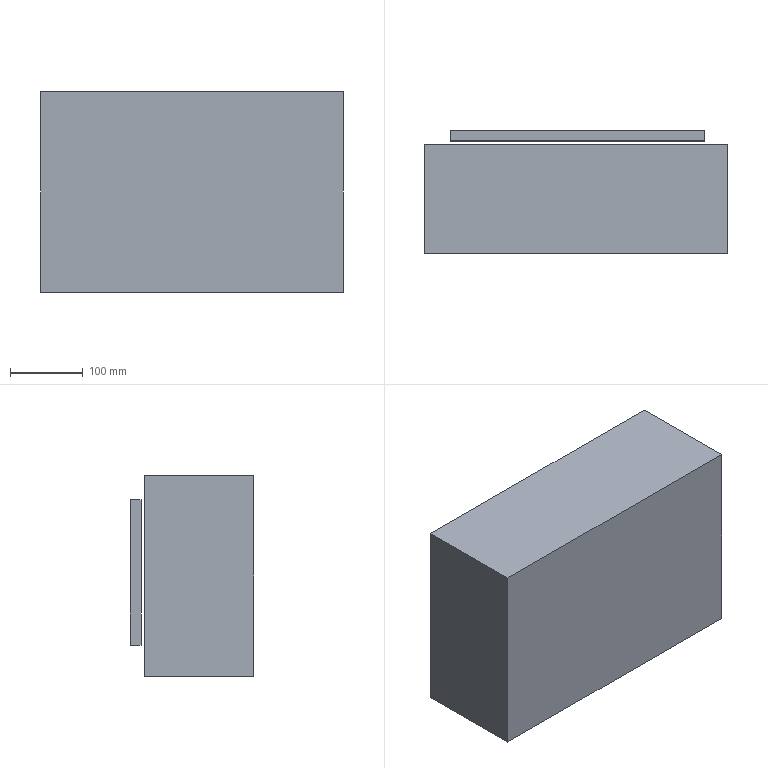Part | STEP file | Plate | 2 solids | 17 faces | box 416 x 170 x 276 mm | volume 18168400 mm3 | plane 17
STEP:
#1=CARTESIAN_POINT('',(0.,0.,0.));
#2=DIRECTION('',(0.,0.,1.));
#3=DIRECTION('',(1.,0.,0.));
#4=AXIS2_PLACEMENT_3D('',#1,#2,#3);
#5=CARTESIAN_POINT('',(238.509,-108.087,0.));
#6=VERTEX_POINT('',#5);
#7=CARTESIAN_POINT('',(238.509,41.913,0.));
#8=VERTEX_POINT('',#7);
#9=CARTESIAN_POINT('',(238.509,-108.087,0.));
#10=DIRECTION('',(0.,1.,0.));
#11=VECTOR('',#10,1.);
#12=LINE('',#9,#11);
#13=CARTESIAN_POINT('',(238.509,-108.087,-276.));
#14=DIRECTION('',(1.,0.,0.));
#15=DIRECTION('',(0.,0.,-1.));
#16=AXIS2_PLACEMENT_3D('',#13,#14,#15);
#17=PLANE('',#16);
#18=CARTESIAN_POINT('',(-276.,0.));
#19=DIRECTION('',(0.,1.));
#20=VECTOR('',#19,1.);
#21=LINE('',#18,#20);
#22=(GEOMETRIC_REPRESENTATION_CONTEXT(2)PARAMETRIC_REPRESENTATION_CONTEXT()REPRESENTATION_CONTEXT('',''));
#23=DEFINITIONAL_REPRESENTATION('',(#21),#22);
#24=PCURVE('',#17,#23);
#25=CARTESIAN_POINT('',(0.,0.,0.));
#26=DIRECTION('',(0.,0.,-1.));
#27=DIRECTION('',(-1.,0.,0.));
#28=AXIS2_PLACEMENT_3D('',#25,#26,#27);
#29=PLANE('',#28);
#30=CARTESIAN_POINT('',(-238.509,-108.087));
#31=DIRECTION('',(0.,1.));
#32=VECTOR('',#31,1.);
#33=LINE('',#30,#32);
#34=(GEOMETRIC_REPRESENTATION_CONTEXT(2)PARAMETRIC_REPRESENTATION_CONTEXT()REPRESENTATION_CONTEXT('',''));
#35=DEFINITIONAL_REPRESENTATION('',(#33),#34);
#36=PCURVE('',#29,#35);
#37=SURFACE_CURVE('',#12,(#24,#36),.PCURVE_S1.);
#38=EDGE_CURVE('',#6,#8,#37,.T.);
#39=ORIENTED_EDGE('',*,*,#38,.F.);
#40=CARTESIAN_POINT('',(238.509,-108.087,-276.));
#41=VERTEX_POINT('',#40);
#42=CARTESIAN_POINT('',(238.509,-108.087,-276.));
#43=DIRECTION('',(0.,0.,1.));
#44=VECTOR('',#43,1.);
#45=LINE('',#42,#44);
#46=CARTESIAN_POINT('',(0.,0.));
#47=DIRECTION('',(-1.,0.));
#48=VECTOR('',#47,1.);
#49=LINE('',#46,#48);
#50=(GEOMETRIC_REPRESENTATION_CONTEXT(2)PARAMETRIC_REPRESENTATION_CONTEXT()REPRESENTATION_CONTEXT('',''));
#51=DEFINITIONAL_REPRESENTATION('',(#49),#50);
#52=PCURVE('',#17,#51);
#53=CARTESIAN_POINT('',(-177.491,-108.087,-276.));
#54=DIRECTION('',(0.,-1.,0.));
#55=DIRECTION('',(0.,0.,-1.));
#56=AXIS2_PLACEMENT_3D('',#53,#54,#55);
#57=PLANE('',#56);
#58=CARTESIAN_POINT('',(0.,416.));
#59=DIRECTION('',(-1.,0.));
#60=VECTOR('',#59,1.);
#61=LINE('',#58,#60);
#62=(GEOMETRIC_REPRESENTATION_CONTEXT(2)PARAMETRIC_REPRESENTATION_CONTEXT()REPRESENTATION_CONTEXT('',''));
#63=DEFINITIONAL_REPRESENTATION('',(#61),#62);
#64=PCURVE('',#57,#63);
#65=SURFACE_CURVE('',#45,(#52,#64),.PCURVE_S1.);
#66=EDGE_CURVE('',#41,#6,#65,.T.);
#67=ORIENTED_EDGE('',*,*,#66,.F.);
#68=CARTESIAN_POINT('',(238.509,41.913,-276.));
#69=VERTEX_POINT('',#68);
#70=CARTESIAN_POINT('',(238.509,-108.087,-276.));
#71=DIRECTION('',(0.,1.,0.));
#72=VECTOR('',#71,1.);
#73=LINE('',#70,#72);
#74=CARTESIAN_POINT('',(0.,0.));
#75=DIRECTION('',(0.,1.));
#76=VECTOR('',#75,1.);
#77=LINE('',#74,#76);
#78=(GEOMETRIC_REPRESENTATION_CONTEXT(2)PARAMETRIC_REPRESENTATION_CONTEXT()REPRESENTATION_CONTEXT('',''));
#79=DEFINITIONAL_REPRESENTATION('',(#77),#78);
#80=PCURVE('',#17,#79);
#81=CARTESIAN_POINT('',(0.,0.,-276.));
#82=DIRECTION('',(0.,0.,-1.));
#83=DIRECTION('',(-1.,0.,0.));
#84=AXIS2_PLACEMENT_3D('',#81,#82,#83);
#85=PLANE('',#84);
#86=CARTESIAN_POINT('',(-238.509,-108.087));
#87=DIRECTION('',(0.,1.));
#88=VECTOR('',#87,1.);
#89=LINE('',#86,#88);
#90=(GEOMETRIC_REPRESENTATION_CONTEXT(2)PARAMETRIC_REPRESENTATION_CONTEXT()REPRESENTATION_CONTEXT('',''));
#91=DEFINITIONAL_REPRESENTATION('',(#89),#90);
#92=PCURVE('',#85,#91);
#93=SURFACE_CURVE('',#73,(#80,#92),.PCURVE_S1.);
#94=EDGE_CURVE('',#41,#69,#93,.T.);
#95=ORIENTED_EDGE('',*,*,#94,.T.);
#96=CARTESIAN_POINT('',(238.509,41.913,-276.));
#97=DIRECTION('',(0.,0.,1.));
#98=VECTOR('',#97,1.);
#99=LINE('',#96,#98);
#100=CARTESIAN_POINT('',(0.,150.));
#101=DIRECTION('',(-1.,0.));
#102=VECTOR('',#101,1.);
#103=LINE('',#100,#102);
#104=(GEOMETRIC_REPRESENTATION_CONTEXT(2)PARAMETRIC_REPRESENTATION_CONTEXT()REPRESENTATION_CONTEXT('',''));
#105=DEFINITIONAL_REPRESENTATION('',(#103),#104);
#106=PCURVE('',#17,#105);
#107=CARTESIAN_POINT('',(-177.491,41.913,-276.));
#108=DIRECTION('',(0.,1.,0.));
#109=DIRECTION('',(0.,0.,1.));
#110=AXIS2_PLACEMENT_3D('',#107,#108,#109);
#111=PLANE('',#110);
#112=CARTESIAN_POINT('',(0.,416.));
#113=DIRECTION('',(1.,0.));
#114=VECTOR('',#113,1.);
#115=LINE('',#112,#114);
#116=(GEOMETRIC_REPRESENTATION_CONTEXT(2)PARAMETRIC_REPRESENTATION_CONTEXT()REPRESENTATION_CONTEXT('',''));
#117=DEFINITIONAL_REPRESENTATION('',(#115),#116);
#118=PCURVE('',#111,#117);
#119=SURFACE_CURVE('',#99,(#106,#118),.PCURVE_S1.);
#120=EDGE_CURVE('',#69,#8,#119,.T.);
#121=ORIENTED_EDGE('',*,*,#120,.T.);
#122=EDGE_LOOP('',(#39,#67,#95,#121));
#123=FACE_BOUND('',#122,.T.);
#124=ADVANCED_FACE('',(#123),#17,.T.);
#125=CARTESIAN_POINT('',(-177.491,-108.087,0.));
#126=VERTEX_POINT('',#125);
#127=CARTESIAN_POINT('',(-177.491,-108.087,0.));
#128=DIRECTION('',(1.,0.,0.));
#129=VECTOR('',#128,1.);
#130=LINE('',#127,#129);
#131=CARTESIAN_POINT('',(-276.,0.));
#132=DIRECTION('',(0.,1.));
#133=VECTOR('',#132,1.);
#134=LINE('',#131,#133);
#135=(GEOMETRIC_REPRESENTATION_CONTEXT(2)PARAMETRIC_REPRESENTATION_CONTEXT()REPRESENTATION_CONTEXT('',''));
#136=DEFINITIONAL_REPRESENTATION('',(#134),#135);
#137=PCURVE('',#57,#136);
#138=CARTESIAN_POINT('',(177.491,-108.087));
#139=DIRECTION('',(-1.,0.));
#140=VECTOR('',#139,1.);
#141=LINE('',#138,#140);
#142=(GEOMETRIC_REPRESENTATION_CONTEXT(2)PARAMETRIC_REPRESENTATION_CONTEXT()REPRESENTATION_CONTEXT('',''));
#143=DEFINITIONAL_REPRESENTATION('',(#141),#142);
#144=PCURVE('',#29,#143);
#145=SURFACE_CURVE('',#130,(#137,#144),.PCURVE_S1.);
#146=EDGE_CURVE('',#126,#6,#145,.T.);
#147=ORIENTED_EDGE('',*,*,#146,.F.);
#148=CARTESIAN_POINT('',(-177.491,-108.087,-276.));
#149=VERTEX_POINT('',#148);
#150=CARTESIAN_POINT('',(-177.491,-108.087,-276.));
#151=DIRECTION('',(0.,0.,1.));
#152=VECTOR('',#151,1.);
#153=LINE('',#150,#152);
#154=CARTESIAN_POINT('',(0.,0.));
#155=DIRECTION('',(-1.,0.));
#156=VECTOR('',#155,1.);
#157=LINE('',#154,#156);
#158=(GEOMETRIC_REPRESENTATION_CONTEXT(2)PARAMETRIC_REPRESENTATION_CONTEXT()REPRESENTATION_CONTEXT('',''));
#159=DEFINITIONAL_REPRESENTATION('',(#157),#158);
#160=PCURVE('',#57,#159);
#161=CARTESIAN_POINT('',(-177.491,-108.087,-276.));
#162=DIRECTION('',(-1.,0.,0.));
#163=DIRECTION('',(0.,0.,1.));
#164=AXIS2_PLACEMENT_3D('',#161,#162,#163);
#165=PLANE('',#164);
#166=CARTESIAN_POINT('',(0.,0.));
#167=DIRECTION('',(1.,0.));
#168=VECTOR('',#167,1.);
#169=LINE('',#166,#168);
#170=(GEOMETRIC_REPRESENTATION_CONTEXT(2)PARAMETRIC_REPRESENTATION_CONTEXT()REPRESENTATION_CONTEXT('',''));
#171=DEFINITIONAL_REPRESENTATION('',(#169),#170);
#172=PCURVE('',#165,#171);
#173=SURFACE_CURVE('',#153,(#160,#172),.PCURVE_S1.);
#174=EDGE_CURVE('',#149,#126,#173,.T.);
#175=ORIENTED_EDGE('',*,*,#174,.F.);
#176=CARTESIAN_POINT('',(-177.491,-108.087,-276.));
#177=DIRECTION('',(1.,0.,0.));
#178=VECTOR('',#177,1.);
#179=LINE('',#176,#178);
#180=CARTESIAN_POINT('',(0.,0.));
#181=DIRECTION('',(0.,1.));
#182=VECTOR('',#181,1.);
#183=LINE('',#180,#182);
#184=(GEOMETRIC_REPRESENTATION_CONTEXT(2)PARAMETRIC_REPRESENTATION_CONTEXT()REPRESENTATION_CONTEXT('',''));
#185=DEFINITIONAL_REPRESENTATION('',(#183),#184);
#186=PCURVE('',#57,#185);
#187=CARTESIAN_POINT('',(177.491,-108.087));
#188=DIRECTION('',(-1.,0.));
#189=VECTOR('',#188,1.);
#190=LINE('',#187,#189);
#191=(GEOMETRIC_REPRESENTATION_CONTEXT(2)PARAMETRIC_REPRESENTATION_CONTEXT()REPRESENTATION_CONTEXT('',''));
#192=DEFINITIONAL_REPRESENTATION('',(#190),#191);
#193=PCURVE('',#85,#192);
#194=SURFACE_CURVE('',#179,(#186,#193),.PCURVE_S1.);
#195=EDGE_CURVE('',#149,#41,#194,.T.);
#196=ORIENTED_EDGE('',*,*,#195,.T.);
#197=ORIENTED_EDGE('',*,*,#66,.T.);
#198=EDGE_LOOP('',(#147,#175,#196,#197));
#199=FACE_BOUND('',#198,.T.);
#200=ADVANCED_FACE('',(#199),#57,.T.);
#201=CARTESIAN_POINT('',(-177.491,41.913,0.));
#202=VERTEX_POINT('',#201);
#203=CARTESIAN_POINT('',(-177.491,-108.087,0.));
#204=DIRECTION('',(0.,-1.,0.));
#205=VECTOR('',#204,1.);
#206=LINE('',#203,#205);
#207=CARTESIAN_POINT('',(276.,0.));
#208=DIRECTION('',(0.,-1.));
#209=VECTOR('',#208,1.);
#210=LINE('',#207,#209);
#211=(GEOMETRIC_REPRESENTATION_CONTEXT(2)PARAMETRIC_REPRESENTATION_CONTEXT()REPRESENTATION_CONTEXT('',''));
#212=DEFINITIONAL_REPRESENTATION('',(#210),#211);
#213=PCURVE('',#165,#212);
#214=CARTESIAN_POINT('',(177.491,-108.087));
#215=DIRECTION('',(0.,-1.));
#216=VECTOR('',#215,1.);
#217=LINE('',#214,#216);
#218=(GEOMETRIC_REPRESENTATION_CONTEXT(2)PARAMETRIC_REPRESENTATION_CONTEXT()REPRESENTATION_CONTEXT('',''));
#219=DEFINITIONAL_REPRESENTATION('',(#217),#218);
#220=PCURVE('',#29,#219);
#221=SURFACE_CURVE('',#206,(#213,#220),.PCURVE_S1.);
#222=EDGE_CURVE('',#202,#126,#221,.T.);
#223=ORIENTED_EDGE('',*,*,#222,.F.);
#224=CARTESIAN_POINT('',(-177.491,41.913,-276.));
#225=VERTEX_POINT('',#224);
#226=CARTESIAN_POINT('',(-177.491,41.913,-276.));
#227=DIRECTION('',(0.,0.,1.));
#228=VECTOR('',#227,1.);
#229=LINE('',#226,#228);
#230=CARTESIAN_POINT('',(0.,150.));
#231=DIRECTION('',(1.,0.));
#232=VECTOR('',#231,1.);
#233=LINE('',#230,#232);
#234=(GEOMETRIC_REPRESENTATION_CONTEXT(2)PARAMETRIC_REPRESENTATION_CONTEXT()REPRESENTATION_CONTEXT('',''));
#235=DEFINITIONAL_REPRESENTATION('',(#233),#234);
#236=PCURVE('',#165,#235);
#237=CARTESIAN_POINT('',(0.,0.));
#238=DIRECTION('',(1.,0.));
#239=VECTOR('',#238,1.);
#240=LINE('',#237,#239);
#241=(GEOMETRIC_REPRESENTATION_CONTEXT(2)PARAMETRIC_REPRESENTATION_CONTEXT()REPRESENTATION_CONTEXT('',''));
#242=DEFINITIONAL_REPRESENTATION('',(#240),#241);
#243=PCURVE('',#111,#242);
#244=SURFACE_CURVE('',#229,(#236,#243),.PCURVE_S1.);
#245=EDGE_CURVE('',#225,#202,#244,.T.);
#246=ORIENTED_EDGE('',*,*,#245,.F.);
#247=CARTESIAN_POINT('',(-177.491,-108.087,-276.));
#248=DIRECTION('',(0.,-1.,0.));
#249=VECTOR('',#248,1.);
#250=LINE('',#247,#249);
#251=CARTESIAN_POINT('',(0.,0.));
#252=DIRECTION('',(0.,-1.));
#253=VECTOR('',#252,1.);
#254=LINE('',#251,#253);
#255=(GEOMETRIC_REPRESENTATION_CONTEXT(2)PARAMETRIC_REPRESENTATION_CONTEXT()REPRESENTATION_CONTEXT('',''));
#256=DEFINITIONAL_REPRESENTATION('',(#254),#255);
#257=PCURVE('',#165,#256);
#258=CARTESIAN_POINT('',(177.491,-108.087));
#259=DIRECTION('',(0.,-1.));
#260=VECTOR('',#259,1.);
#261=LINE('',#258,#260);
#262=(GEOMETRIC_REPRESENTATION_CONTEXT(2)PARAMETRIC_REPRESENTATION_CONTEXT()REPRESENTATION_CONTEXT('',''));
#263=DEFINITIONAL_REPRESENTATION('',(#261),#262);
#264=PCURVE('',#85,#263);
#265=SURFACE_CURVE('',#250,(#257,#264),.PCURVE_S1.);
#266=EDGE_CURVE('',#225,#149,#265,.T.);
#267=ORIENTED_EDGE('',*,*,#266,.T.);
#268=ORIENTED_EDGE('',*,*,#174,.T.);
#269=EDGE_LOOP('',(#223,#246,#267,#268));
#270=FACE_BOUND('',#269,.T.);
#271=ADVANCED_FACE('',(#270),#165,.T.);
#272=CARTESIAN_POINT('',(-169.491,41.913,-268.));
#273=VERTEX_POINT('',#272);
#274=CARTESIAN_POINT('',(-169.491,41.913,-8.));
#275=VERTEX_POINT('',#274);
#276=CARTESIAN_POINT('',(-169.491,41.913,-8.));
#277=DIRECTION('',(0.,0.,1.));
#278=VECTOR('',#277,1.);
#279=LINE('',#276,#278);
#280=CARTESIAN_POINT('',(268.,8.));
#281=DIRECTION('',(1.,0.));
#282=VECTOR('',#281,1.);
#283=LINE('',#280,#282);
#284=(GEOMETRIC_REPRESENTATION_CONTEXT(2)PARAMETRIC_REPRESENTATION_CONTEXT()REPRESENTATION_CONTEXT('',''));
#285=DEFINITIONAL_REPRESENTATION('',(#283),#284);
#286=PCURVE('',#111,#285);
#287=CARTESIAN_POINT('',(-169.491,40.913,-8.));
#288=DIRECTION('',(-1.,0.,0.));
#289=DIRECTION('',(0.,0.,1.));
#290=AXIS2_PLACEMENT_3D('',#287,#288,#289);
#291=PLANE('',#290);
#292=CARTESIAN_POINT('',(0.,1.));
#293=DIRECTION('',(1.,0.));
#294=VECTOR('',#293,1.);
#295=LINE('',#292,#294);
#296=(GEOMETRIC_REPRESENTATION_CONTEXT(2)PARAMETRIC_REPRESENTATION_CONTEXT()REPRESENTATION_CONTEXT('',''));
#297=DEFINITIONAL_REPRESENTATION('',(#295),#296);
#298=PCURVE('',#291,#297);
#299=SURFACE_CURVE('',#279,(#286,#298),.PCURVE_S1.);
#300=EDGE_CURVE('',#273,#275,#299,.T.);
#301=ORIENTED_EDGE('',*,*,#300,.F.);
#302=CARTESIAN_POINT('',(230.509,41.913,-268.));
#303=VERTEX_POINT('',#302);
#304=CARTESIAN_POINT('',(-169.491,41.913,-268.));
#305=DIRECTION('',(-1.,0.,0.));
#306=VECTOR('',#305,1.);
#307=LINE('',#304,#306);
#308=CARTESIAN_POINT('',(8.,8.));
#309=DIRECTION('',(0.,-1.));
#310=VECTOR('',#309,1.);
#311=LINE('',#308,#310);
#312=(GEOMETRIC_REPRESENTATION_CONTEXT(2)PARAMETRIC_REPRESENTATION_CONTEXT()REPRESENTATION_CONTEXT('',''));
#313=DEFINITIONAL_REPRESENTATION('',(#311),#312);
#314=PCURVE('',#111,#313);
#315=CARTESIAN_POINT('',(-169.491,40.913,-268.));
#316=DIRECTION('',(0.,0.,-1.));
#317=DIRECTION('',(-1.,0.,0.));
#318=AXIS2_PLACEMENT_3D('',#315,#316,#317);
#319=PLANE('',#318);
#320=CARTESIAN_POINT('',(0.,1.));
#321=DIRECTION('',(1.,0.));
#322=VECTOR('',#321,1.);
#323=LINE('',#320,#322);
#324=(GEOMETRIC_REPRESENTATION_CONTEXT(2)PARAMETRIC_REPRESENTATION_CONTEXT()REPRESENTATION_CONTEXT('',''));
#325=DEFINITIONAL_REPRESENTATION('',(#323),#324);
#326=PCURVE('',#319,#325);
#327=SURFACE_CURVE('',#307,(#314,#326),.PCURVE_S1.);
#328=EDGE_CURVE('',#303,#273,#327,.T.);
#329=ORIENTED_EDGE('',*,*,#328,.F.);
#330=CARTESIAN_POINT('',(230.509,41.913,-8.));
#331=VERTEX_POINT('',#330);
#332=CARTESIAN_POINT('',(230.509,41.913,-8.));
#333=DIRECTION('',(0.,0.,-1.));
#334=VECTOR('',#333,1.);
#335=LINE('',#332,#334);
#336=CARTESIAN_POINT('',(268.,408.));
#337=DIRECTION('',(-1.,0.));
#338=VECTOR('',#337,1.);
#339=LINE('',#336,#338);
#340=(GEOMETRIC_REPRESENTATION_CONTEXT(2)PARAMETRIC_REPRESENTATION_CONTEXT()REPRESENTATION_CONTEXT('',''));
#341=DEFINITIONAL_REPRESENTATION('',(#339),#340);
#342=PCURVE('',#111,#341);
#343=CARTESIAN_POINT('',(230.509,40.913,-8.));
#344=DIRECTION('',(1.,0.,0.));
#345=DIRECTION('',(0.,0.,-1.));
#346=AXIS2_PLACEMENT_3D('',#343,#344,#345);
#347=PLANE('',#346);
#348=CARTESIAN_POINT('',(0.,1.));
#349=DIRECTION('',(1.,0.));
#350=VECTOR('',#349,1.);
#351=LINE('',#348,#350);
#352=(GEOMETRIC_REPRESENTATION_CONTEXT(2)PARAMETRIC_REPRESENTATION_CONTEXT()REPRESENTATION_CONTEXT('',''));
#353=DEFINITIONAL_REPRESENTATION('',(#351),#352);
#354=PCURVE('',#347,#353);
#355=SURFACE_CURVE('',#335,(#342,#354),.PCURVE_S1.);
#356=EDGE_CURVE('',#331,#303,#355,.T.);
#357=ORIENTED_EDGE('',*,*,#356,.F.);
#358=CARTESIAN_POINT('',(-169.491,41.913,-8.));
#359=DIRECTION('',(1.,0.,0.));
#360=VECTOR('',#359,1.);
#361=LINE('',#358,#360);
#362=CARTESIAN_POINT('',(268.,8.));
#363=DIRECTION('',(0.,1.));
#364=VECTOR('',#363,1.);
#365=LINE('',#362,#364);
#366=(GEOMETRIC_REPRESENTATION_CONTEXT(2)PARAMETRIC_REPRESENTATION_CONTEXT()REPRESENTATION_CONTEXT('',''));
#367=DEFINITIONAL_REPRESENTATION('',(#365),#366);
#368=PCURVE('',#111,#367);
#369=CARTESIAN_POINT('',(-169.491,40.913,-8.));
#370=DIRECTION('',(0.,0.,1.));
#371=DIRECTION('',(1.,0.,0.));
#372=AXIS2_PLACEMENT_3D('',#369,#370,#371);
#373=PLANE('',#372);
#374=CARTESIAN_POINT('',(0.,1.));
#375=DIRECTION('',(1.,0.));
#376=VECTOR('',#375,1.);
#377=LINE('',#374,#376);
#378=(GEOMETRIC_REPRESENTATION_CONTEXT(2)PARAMETRIC_REPRESENTATION_CONTEXT()REPRESENTATION_CONTEXT('',''));
#379=DEFINITIONAL_REPRESENTATION('',(#377),#378);
#380=PCURVE('',#373,#379);
#381=SURFACE_CURVE('',#361,(#368,#380),.PCURVE_S1.);
#382=EDGE_CURVE('',#275,#331,#381,.T.);
#383=ORIENTED_EDGE('',*,*,#382,.F.);
#384=EDGE_LOOP('',(#301,#329,#357,#383));
#385=FACE_BOUND('',#384,.T.);
#386=CARTESIAN_POINT('',(-177.491,41.913,0.));
#387=DIRECTION('',(-1.,0.,0.));
#388=VECTOR('',#387,1.);
#389=LINE('',#386,#388);
#390=CARTESIAN_POINT('',(276.,0.));
#391=DIRECTION('',(0.,-1.));
#392=VECTOR('',#391,1.);
#393=LINE('',#390,#392);
#394=(GEOMETRIC_REPRESENTATION_CONTEXT(2)PARAMETRIC_REPRESENTATION_CONTEXT()REPRESENTATION_CONTEXT('',''));
#395=DEFINITIONAL_REPRESENTATION('',(#393),#394);
#396=PCURVE('',#111,#395);
#397=CARTESIAN_POINT('',(177.491,41.913));
#398=DIRECTION('',(1.,0.));
#399=VECTOR('',#398,1.);
#400=LINE('',#397,#399);
#401=(GEOMETRIC_REPRESENTATION_CONTEXT(2)PARAMETRIC_REPRESENTATION_CONTEXT()REPRESENTATION_CONTEXT('',''));
#402=DEFINITIONAL_REPRESENTATION('',(#400),#401);
#403=PCURVE('',#29,#402);
#404=SURFACE_CURVE('',#389,(#396,#403),.PCURVE_S1.);
#405=EDGE_CURVE('',#8,#202,#404,.T.);
#406=ORIENTED_EDGE('',*,*,#405,.F.);
#407=ORIENTED_EDGE('',*,*,#120,.F.);
#408=CARTESIAN_POINT('',(-177.491,41.913,-276.));
#409=DIRECTION('',(-1.,0.,0.));
#410=VECTOR('',#409,1.);
#411=LINE('',#408,#410);
#412=CARTESIAN_POINT('',(0.,0.));
#413=DIRECTION('',(0.,-1.));
#414=VECTOR('',#413,1.);
#415=LINE('',#412,#414);
#416=(GEOMETRIC_REPRESENTATION_CONTEXT(2)PARAMETRIC_REPRESENTATION_CONTEXT()REPRESENTATION_CONTEXT('',''));
#417=DEFINITIONAL_REPRESENTATION('',(#415),#416);
#418=PCURVE('',#111,#417);
#419=CARTESIAN_POINT('',(177.491,41.913));
#420=DIRECTION('',(1.,0.));
#421=VECTOR('',#420,1.);
#422=LINE('',#419,#421);
#423=(GEOMETRIC_REPRESENTATION_CONTEXT(2)PARAMETRIC_REPRESENTATION_CONTEXT()REPRESENTATION_CONTEXT('',''));
#424=DEFINITIONAL_REPRESENTATION('',(#422),#423);
#425=PCURVE('',#85,#424);
#426=SURFACE_CURVE('',#411,(#418,#425),.PCURVE_S1.);
#427=EDGE_CURVE('',#69,#225,#426,.T.);
#428=ORIENTED_EDGE('',*,*,#427,.T.);
#429=ORIENTED_EDGE('',*,*,#245,.T.);
#430=EDGE_LOOP('',(#406,#407,#428,#429));
#431=FACE_BOUND('',#430,.T.);
#432=ADVANCED_FACE('',(#385,#431),#111,.T.);
#433=ORIENTED_EDGE('',*,*,#94,.F.);
#434=ORIENTED_EDGE('',*,*,#195,.F.);
#435=ORIENTED_EDGE('',*,*,#266,.F.);
#436=ORIENTED_EDGE('',*,*,#427,.F.);
#437=EDGE_LOOP('',(#433,#434,#435,#436));
#438=FACE_BOUND('',#437,.T.);
#439=ADVANCED_FACE('',(#438),#85,.T.);
#440=ORIENTED_EDGE('',*,*,#38,.T.);
#441=ORIENTED_EDGE('',*,*,#405,.T.);
#442=ORIENTED_EDGE('',*,*,#222,.T.);
#443=ORIENTED_EDGE('',*,*,#146,.T.);
#444=EDGE_LOOP('',(#440,#441,#442,#443));
#445=FACE_BOUND('',#444,.T.);
#446=ADVANCED_FACE('',(#445),#29,.F.);
#447=ORIENTED_EDGE('',*,*,#300,.T.);
#448=CARTESIAN_POINT('',(-169.491,40.913,-8.));
#449=VERTEX_POINT('',#448);
#450=CARTESIAN_POINT('',(-169.491,40.913,-8.));
#451=DIRECTION('',(0.,1.,0.));
#452=VECTOR('',#451,1.);
#453=LINE('',#450,#452);
#454=CARTESIAN_POINT('',(0.,0.));
#455=DIRECTION('',(0.,1.));
#456=VECTOR('',#455,1.);
#457=LINE('',#454,#456);
#458=(GEOMETRIC_REPRESENTATION_CONTEXT(2)PARAMETRIC_REPRESENTATION_CONTEXT()REPRESENTATION_CONTEXT('',''));
#459=DEFINITIONAL_REPRESENTATION('',(#457),#458);
#460=PCURVE('',#291,#459);
#461=CARTESIAN_POINT('',(0.,0.));
#462=DIRECTION('',(0.,1.));
#463=VECTOR('',#462,1.);
#464=LINE('',#461,#463);
#465=(GEOMETRIC_REPRESENTATION_CONTEXT(2)PARAMETRIC_REPRESENTATION_CONTEXT()REPRESENTATION_CONTEXT('',''));
#466=DEFINITIONAL_REPRESENTATION('',(#464),#465);
#467=PCURVE('',#373,#466);
#468=SURFACE_CURVE('',#453,(#460,#467),.PCURVE_S1.);
#469=EDGE_CURVE('',#449,#275,#468,.T.);
#470=ORIENTED_EDGE('',*,*,#469,.F.);
#471=CARTESIAN_POINT('',(-169.491,40.913,-268.));
#472=VERTEX_POINT('',#471);
#473=CARTESIAN_POINT('',(-169.491,40.913,-8.));
#474=DIRECTION('',(0.,0.,1.));
#475=VECTOR('',#474,1.);
#476=LINE('',#473,#475);
#477=CARTESIAN_POINT('',(0.,0.));
#478=DIRECTION('',(1.,0.));
#479=VECTOR('',#478,1.);
#480=LINE('',#477,#479);
#481=(GEOMETRIC_REPRESENTATION_CONTEXT(2)PARAMETRIC_REPRESENTATION_CONTEXT()REPRESENTATION_CONTEXT('',''));
#482=DEFINITIONAL_REPRESENTATION('',(#480),#481);
#483=PCURVE('',#291,#482);
#484=CARTESIAN_POINT('',(0.,40.913,0.));
#485=DIRECTION('',(0.,-1.,0.));
#486=DIRECTION('',(0.,0.,-1.));
#487=AXIS2_PLACEMENT_3D('',#484,#485,#486);
#488=PLANE('',#487);
#489=CARTESIAN_POINT('',(8.,-169.491));
#490=DIRECTION('',(-1.,0.));
#491=VECTOR('',#490,1.);
#492=LINE('',#489,#491);
#493=(GEOMETRIC_REPRESENTATION_CONTEXT(2)PARAMETRIC_REPRESENTATION_CONTEXT()REPRESENTATION_CONTEXT('',''));
#494=DEFINITIONAL_REPRESENTATION('',(#492),#493);
#495=PCURVE('',#488,#494);
#496=SURFACE_CURVE('',#476,(#483,#495),.PCURVE_S1.);
#497=EDGE_CURVE('',#472,#449,#496,.T.);
#498=ORIENTED_EDGE('',*,*,#497,.F.);
#499=CARTESIAN_POINT('',(-169.491,40.913,-268.));
#500=DIRECTION('',(0.,1.,0.));
#501=VECTOR('',#500,1.);
#502=LINE('',#499,#501);
#503=CARTESIAN_POINT('',(-260.,0.));
#504=DIRECTION('',(0.,1.));
#505=VECTOR('',#504,1.);
#506=LINE('',#503,#505);
#507=(GEOMETRIC_REPRESENTATION_CONTEXT(2)PARAMETRIC_REPRESENTATION_CONTEXT()REPRESENTATION_CONTEXT('',''));
#508=DEFINITIONAL_REPRESENTATION('',(#506),#507);
#509=PCURVE('',#291,#508);
#510=CARTESIAN_POINT('',(0.,0.));
#511=DIRECTION('',(0.,1.));
#512=VECTOR('',#511,1.);
#513=LINE('',#510,#512);
#514=(GEOMETRIC_REPRESENTATION_CONTEXT(2)PARAMETRIC_REPRESENTATION_CONTEXT()REPRESENTATION_CONTEXT('',''));
#515=DEFINITIONAL_REPRESENTATION('',(#513),#514);
#516=PCURVE('',#319,#515);
#517=SURFACE_CURVE('',#502,(#509,#516),.PCURVE_S1.);
#518=EDGE_CURVE('',#472,#273,#517,.T.);
#519=ORIENTED_EDGE('',*,*,#518,.T.);
#520=EDGE_LOOP('',(#447,#470,#498,#519));
#521=FACE_BOUND('',#520,.T.);
#522=ADVANCED_FACE('',(#521),#291,.F.);
#523=ORIENTED_EDGE('',*,*,#328,.T.);
#524=ORIENTED_EDGE('',*,*,#518,.F.);
#525=CARTESIAN_POINT('',(230.509,40.913,-268.));
#526=VERTEX_POINT('',#525);
#527=CARTESIAN_POINT('',(-169.491,40.913,-268.));
#528=DIRECTION('',(-1.,0.,0.));
#529=VECTOR('',#528,1.);
#530=LINE('',#527,#529);
#531=CARTESIAN_POINT('',(0.,0.));
#532=DIRECTION('',(1.,0.));
#533=VECTOR('',#532,1.);
#534=LINE('',#531,#533);
#535=(GEOMETRIC_REPRESENTATION_CONTEXT(2)PARAMETRIC_REPRESENTATION_CONTEXT()REPRESENTATION_CONTEXT('',''));
#536=DEFINITIONAL_REPRESENTATION('',(#534),#535);
#537=PCURVE('',#319,#536);
#538=CARTESIAN_POINT('',(268.,-169.491));
#539=DIRECTION('',(0.,-1.));
#540=VECTOR('',#539,1.);
#541=LINE('',#538,#540);
#542=(GEOMETRIC_REPRESENTATION_CONTEXT(2)PARAMETRIC_REPRESENTATION_CONTEXT()REPRESENTATION_CONTEXT('',''));
#543=DEFINITIONAL_REPRESENTATION('',(#541),#542);
#544=PCURVE('',#488,#543);
#545=SURFACE_CURVE('',#530,(#537,#544),.PCURVE_S1.);
#546=EDGE_CURVE('',#526,#472,#545,.T.);
#547=ORIENTED_EDGE('',*,*,#546,.F.);
#548=CARTESIAN_POINT('',(230.509,40.913,-268.));
#549=DIRECTION('',(0.,1.,0.));
#550=VECTOR('',#549,1.);
#551=LINE('',#548,#550);
#552=CARTESIAN_POINT('',(-400.,0.));
#553=DIRECTION('',(0.,1.));
#554=VECTOR('',#553,1.);
#555=LINE('',#552,#554);
#556=(GEOMETRIC_REPRESENTATION_CONTEXT(2)PARAMETRIC_REPRESENTATION_CONTEXT()REPRESENTATION_CONTEXT('',''));
#557=DEFINITIONAL_REPRESENTATION('',(#555),#556);
#558=PCURVE('',#319,#557);
#559=CARTESIAN_POINT('',(260.,0.));
#560=DIRECTION('',(0.,1.));
#561=VECTOR('',#560,1.);
#562=LINE('',#559,#561);
#563=(GEOMETRIC_REPRESENTATION_CONTEXT(2)PARAMETRIC_REPRESENTATION_CONTEXT()REPRESENTATION_CONTEXT('',''));
#564=DEFINITIONAL_REPRESENTATION('',(#562),#563);
#565=PCURVE('',#347,#564);
#566=SURFACE_CURVE('',#551,(#558,#565),.PCURVE_S1.);
#567=EDGE_CURVE('',#526,#303,#566,.T.);
#568=ORIENTED_EDGE('',*,*,#567,.T.);
#569=EDGE_LOOP('',(#523,#524,#547,#568));
#570=FACE_BOUND('',#569,.T.);
#571=ADVANCED_FACE('',(#570),#319,.F.);
#572=ORIENTED_EDGE('',*,*,#356,.T.);
#573=ORIENTED_EDGE('',*,*,#567,.F.);
#574=CARTESIAN_POINT('',(230.509,40.913,-8.));
#575=VERTEX_POINT('',#574);
#576=CARTESIAN_POINT('',(230.509,40.913,-8.));
#577=DIRECTION('',(0.,0.,-1.));
#578=VECTOR('',#577,1.);
#579=LINE('',#576,#578);
#580=CARTESIAN_POINT('',(0.,0.));
#581=DIRECTION('',(1.,0.));
#582=VECTOR('',#581,1.);
#583=LINE('',#580,#582);
#584=(GEOMETRIC_REPRESENTATION_CONTEXT(2)PARAMETRIC_REPRESENTATION_CONTEXT()REPRESENTATION_CONTEXT('',''));
#585=DEFINITIONAL_REPRESENTATION('',(#583),#584);
#586=PCURVE('',#347,#585);
#587=CARTESIAN_POINT('',(8.,230.509));
#588=DIRECTION('',(1.,0.));
#589=VECTOR('',#588,1.);
#590=LINE('',#587,#589);
#591=(GEOMETRIC_REPRESENTATION_CONTEXT(2)PARAMETRIC_REPRESENTATION_CONTEXT()REPRESENTATION_CONTEXT('',''));
#592=DEFINITIONAL_REPRESENTATION('',(#590),#591);
#593=PCURVE('',#488,#592);
#594=SURFACE_CURVE('',#579,(#586,#593),.PCURVE_S1.);
#595=EDGE_CURVE('',#575,#526,#594,.T.);
#596=ORIENTED_EDGE('',*,*,#595,.F.);
#597=CARTESIAN_POINT('',(230.509,40.913,-8.));
#598=DIRECTION('',(0.,1.,0.));
#599=VECTOR('',#598,1.);
#600=LINE('',#597,#599);
#601=CARTESIAN_POINT('',(0.,0.));
#602=DIRECTION('',(0.,1.));
#603=VECTOR('',#602,1.);
#604=LINE('',#601,#603);
#605=(GEOMETRIC_REPRESENTATION_CONTEXT(2)PARAMETRIC_REPRESENTATION_CONTEXT()REPRESENTATION_CONTEXT('',''));
#606=DEFINITIONAL_REPRESENTATION('',(#604),#605);
#607=PCURVE('',#347,#606);
#608=CARTESIAN_POINT('',(400.,0.));
#609=DIRECTION('',(0.,1.));
#610=VECTOR('',#609,1.);
#611=LINE('',#608,#610);
#612=(GEOMETRIC_REPRESENTATION_CONTEXT(2)PARAMETRIC_REPRESENTATION_CONTEXT()REPRESENTATION_CONTEXT('',''));
#613=DEFINITIONAL_REPRESENTATION('',(#611),#612);
#614=PCURVE('',#373,#613);
#615=SURFACE_CURVE('',#600,(#607,#614),.PCURVE_S1.);
#616=EDGE_CURVE('',#575,#331,#615,.T.);
#617=ORIENTED_EDGE('',*,*,#616,.T.);
#618=EDGE_LOOP('',(#572,#573,#596,#617));
#619=FACE_BOUND('',#618,.T.);
#620=ADVANCED_FACE('',(#619),#347,.F.);
#621=ORIENTED_EDGE('',*,*,#382,.T.);
#622=ORIENTED_EDGE('',*,*,#616,.F.);
#623=CARTESIAN_POINT('',(-169.491,40.913,-8.));
#624=DIRECTION('',(1.,0.,0.));
#625=VECTOR('',#624,1.);
#626=LINE('',#623,#625);
#627=CARTESIAN_POINT('',(0.,0.));
#628=DIRECTION('',(1.,0.));
#629=VECTOR('',#628,1.);
#630=LINE('',#627,#629);
#631=(GEOMETRIC_REPRESENTATION_CONTEXT(2)PARAMETRIC_REPRESENTATION_CONTEXT()REPRESENTATION_CONTEXT('',''));
#632=DEFINITIONAL_REPRESENTATION('',(#630),#631);
#633=PCURVE('',#373,#632);
#634=CARTESIAN_POINT('',(8.,-169.491));
#635=DIRECTION('',(0.,1.));
#636=VECTOR('',#635,1.);
#637=LINE('',#634,#636);
#638=(GEOMETRIC_REPRESENTATION_CONTEXT(2)PARAMETRIC_REPRESENTATION_CONTEXT()REPRESENTATION_CONTEXT('',''));
#639=DEFINITIONAL_REPRESENTATION('',(#637),#638);
#640=PCURVE('',#488,#639);
#641=SURFACE_CURVE('',#626,(#633,#640),.PCURVE_S1.);
#642=EDGE_CURVE('',#449,#575,#641,.T.);
#643=ORIENTED_EDGE('',*,*,#642,.F.);
#644=ORIENTED_EDGE('',*,*,#469,.T.);
#645=EDGE_LOOP('',(#621,#622,#643,#644));
#646=FACE_BOUND('',#645,.T.);
#647=ADVANCED_FACE('',(#646),#373,.F.);
#648=ORIENTED_EDGE('',*,*,#497,.T.);
#649=ORIENTED_EDGE('',*,*,#642,.T.);
#650=ORIENTED_EDGE('',*,*,#595,.T.);
#651=ORIENTED_EDGE('',*,*,#546,.T.);
#652=EDGE_LOOP('',(#648,#649,#650,#651));
#653=FACE_BOUND('',#652,.T.);
#654=ADVANCED_FACE('',(#653),#488,.F.);
#655=CLOSED_SHELL('',(#124,#200,#271,#432,#439,#446,#522,#571,#620,#647,#654));
#656=MANIFOLD_SOLID_BREP('',#655);
#657=CARTESIAN_POINT('',(-142.491,61.913,-33.));
#658=VERTEX_POINT('',#657);
#659=CARTESIAN_POINT('',(207.509,61.913,-33.));
#660=VERTEX_POINT('',#659);
#661=CARTESIAN_POINT('',(-142.491,61.913,-33.));
#662=DIRECTION('',(1.,0.,0.));
#663=VECTOR('',#662,1.);
#664=LINE('',#661,#663);
#665=CARTESIAN_POINT('',(-142.491,46.913,-33.));
#666=DIRECTION('',(0.,0.,1.));
#667=DIRECTION('',(1.,0.,0.));
#668=AXIS2_PLACEMENT_3D('',#665,#666,#667);
#669=PLANE('',#668);
#670=CARTESIAN_POINT('',(0.,15.));
#671=DIRECTION('',(1.,0.));
#672=VECTOR('',#671,1.);
#673=LINE('',#670,#672);
#674=(GEOMETRIC_REPRESENTATION_CONTEXT(2)PARAMETRIC_REPRESENTATION_CONTEXT()REPRESENTATION_CONTEXT('',''));
#675=DEFINITIONAL_REPRESENTATION('',(#673),#674);
#676=PCURVE('',#669,#675);
#677=CARTESIAN_POINT('',(0.,61.913,0.));
#678=DIRECTION('',(0.,1.,0.));
#679=DIRECTION('',(0.,0.,1.));
#680=AXIS2_PLACEMENT_3D('',#677,#678,#679);
#681=PLANE('',#680);
#682=CARTESIAN_POINT('',(-33.,-142.491));
#683=DIRECTION('',(0.,1.));
#684=VECTOR('',#683,1.);
#685=LINE('',#682,#684);
#686=(GEOMETRIC_REPRESENTATION_CONTEXT(2)PARAMETRIC_REPRESENTATION_CONTEXT()REPRESENTATION_CONTEXT('',''));
#687=DEFINITIONAL_REPRESENTATION('',(#685),#686);
#688=PCURVE('',#681,#687);
#689=SURFACE_CURVE('',#664,(#676,#688),.PCURVE_S1.);
#690=EDGE_CURVE('',#658,#660,#689,.T.);
#691=ORIENTED_EDGE('',*,*,#690,.F.);
#692=CARTESIAN_POINT('',(-142.491,46.913,-33.));
#693=VERTEX_POINT('',#692);
#694=CARTESIAN_POINT('',(-142.491,46.913,-33.));
#695=DIRECTION('',(0.,1.,0.));
#696=VECTOR('',#695,1.);
#697=LINE('',#694,#696);
#698=CARTESIAN_POINT('',(0.,0.));
#699=DIRECTION('',(0.,1.));
#700=VECTOR('',#699,1.);
#701=LINE('',#698,#700);
#702=(GEOMETRIC_REPRESENTATION_CONTEXT(2)PARAMETRIC_REPRESENTATION_CONTEXT()REPRESENTATION_CONTEXT('',''));
#703=DEFINITIONAL_REPRESENTATION('',(#701),#702);
#704=PCURVE('',#669,#703);
#705=CARTESIAN_POINT('',(-142.491,46.913,-33.));
#706=DIRECTION('',(-1.,0.,0.));
#707=DIRECTION('',(0.,0.,1.));
#708=AXIS2_PLACEMENT_3D('',#705,#706,#707);
#709=PLANE('',#708);
#710=CARTESIAN_POINT('',(0.,0.));
#711=DIRECTION('',(0.,1.));
#712=VECTOR('',#711,1.);
#713=LINE('',#710,#712);
#714=(GEOMETRIC_REPRESENTATION_CONTEXT(2)PARAMETRIC_REPRESENTATION_CONTEXT()REPRESENTATION_CONTEXT('',''));
#715=DEFINITIONAL_REPRESENTATION('',(#713),#714);
#716=PCURVE('',#709,#715);
#717=SURFACE_CURVE('',#697,(#704,#716),.PCURVE_S1.);
#718=EDGE_CURVE('',#693,#658,#717,.T.);
#719=ORIENTED_EDGE('',*,*,#718,.F.);
#720=CARTESIAN_POINT('',(207.509,46.913,-33.));
#721=VERTEX_POINT('',#720);
#722=CARTESIAN_POINT('',(-142.491,46.913,-33.));
#723=DIRECTION('',(1.,0.,0.));
#724=VECTOR('',#723,1.);
#725=LINE('',#722,#724);
#726=CARTESIAN_POINT('',(0.,0.));
#727=DIRECTION('',(1.,0.));
#728=VECTOR('',#727,1.);
#729=LINE('',#726,#728);
#730=(GEOMETRIC_REPRESENTATION_CONTEXT(2)PARAMETRIC_REPRESENTATION_CONTEXT()REPRESENTATION_CONTEXT('',''));
#731=DEFINITIONAL_REPRESENTATION('',(#729),#730);
#732=PCURVE('',#669,#731);
#733=CARTESIAN_POINT('',(0.,46.913,0.));
#734=DIRECTION('',(0.,1.,0.));
#735=DIRECTION('',(0.,0.,1.));
#736=AXIS2_PLACEMENT_3D('',#733,#734,#735);
#737=PLANE('',#736);
#738=CARTESIAN_POINT('',(-33.,-142.491));
#739=DIRECTION('',(0.,1.));
#740=VECTOR('',#739,1.);
#741=LINE('',#738,#740);
#742=(GEOMETRIC_REPRESENTATION_CONTEXT(2)PARAMETRIC_REPRESENTATION_CONTEXT()REPRESENTATION_CONTEXT('',''));
#743=DEFINITIONAL_REPRESENTATION('',(#741),#742);
#744=PCURVE('',#737,#743);
#745=SURFACE_CURVE('',#725,(#732,#744),.PCURVE_S1.);
#746=EDGE_CURVE('',#693,#721,#745,.T.);
#747=ORIENTED_EDGE('',*,*,#746,.T.);
#748=CARTESIAN_POINT('',(207.509,46.913,-33.));
#749=DIRECTION('',(0.,1.,0.));
#750=VECTOR('',#749,1.);
#751=LINE('',#748,#750);
#752=CARTESIAN_POINT('',(350.,0.));
#753=DIRECTION('',(0.,1.));
#754=VECTOR('',#753,1.);
#755=LINE('',#752,#754);
#756=(GEOMETRIC_REPRESENTATION_CONTEXT(2)PARAMETRIC_REPRESENTATION_CONTEXT()REPRESENTATION_CONTEXT('',''));
#757=DEFINITIONAL_REPRESENTATION('',(#755),#756);
#758=PCURVE('',#669,#757);
#759=CARTESIAN_POINT('',(207.509,46.913,-33.));
#760=DIRECTION('',(1.,0.,0.));
#761=DIRECTION('',(0.,0.,-1.));
#762=AXIS2_PLACEMENT_3D('',#759,#760,#761);
#763=PLANE('',#762);
#764=CARTESIAN_POINT('',(0.,0.));
#765=DIRECTION('',(0.,1.));
#766=VECTOR('',#765,1.);
#767=LINE('',#764,#766);
#768=(GEOMETRIC_REPRESENTATION_CONTEXT(2)PARAMETRIC_REPRESENTATION_CONTEXT()REPRESENTATION_CONTEXT('',''));
#769=DEFINITIONAL_REPRESENTATION('',(#767),#768);
#770=PCURVE('',#763,#769);
#771=SURFACE_CURVE('',#751,(#758,#770),.PCURVE_S1.);
#772=EDGE_CURVE('',#721,#660,#771,.T.);
#773=ORIENTED_EDGE('',*,*,#772,.T.);
#774=EDGE_LOOP('',(#691,#719,#747,#773));
#775=FACE_BOUND('',#774,.T.);
#776=ADVANCED_FACE('',(#775),#669,.T.);
#777=CARTESIAN_POINT('',(-142.491,61.913,-233.));
#778=VERTEX_POINT('',#777);
#779=CARTESIAN_POINT('',(-142.491,61.913,-33.));
#780=DIRECTION('',(0.,0.,1.));
#781=VECTOR('',#780,1.);
#782=LINE('',#779,#781);
#783=CARTESIAN_POINT('',(0.,15.));
#784=DIRECTION('',(1.,0.));
#785=VECTOR('',#784,1.);
#786=LINE('',#783,#785);
#787=(GEOMETRIC_REPRESENTATION_CONTEXT(2)PARAMETRIC_REPRESENTATION_CONTEXT()REPRESENTATION_CONTEXT('',''));
#788=DEFINITIONAL_REPRESENTATION('',(#786),#787);
#789=PCURVE('',#709,#788);
#790=CARTESIAN_POINT('',(-33.,-142.491));
#791=DIRECTION('',(1.,0.));
#792=VECTOR('',#791,1.);
#793=LINE('',#790,#792);
#794=(GEOMETRIC_REPRESENTATION_CONTEXT(2)PARAMETRIC_REPRESENTATION_CONTEXT()REPRESENTATION_CONTEXT('',''));
#795=DEFINITIONAL_REPRESENTATION('',(#793),#794);
#796=PCURVE('',#681,#795);
#797=SURFACE_CURVE('',#782,(#789,#796),.PCURVE_S1.);
#798=EDGE_CURVE('',#778,#658,#797,.T.);
#799=ORIENTED_EDGE('',*,*,#798,.F.);
#800=CARTESIAN_POINT('',(-142.491,46.913,-233.));
#801=VERTEX_POINT('',#800);
#802=CARTESIAN_POINT('',(-142.491,46.913,-233.));
#803=DIRECTION('',(0.,1.,0.));
#804=VECTOR('',#803,1.);
#805=LINE('',#802,#804);
#806=CARTESIAN_POINT('',(-200.,0.));
#807=DIRECTION('',(0.,1.));
#808=VECTOR('',#807,1.);
#809=LINE('',#806,#808);
#810=(GEOMETRIC_REPRESENTATION_CONTEXT(2)PARAMETRIC_REPRESENTATION_CONTEXT()REPRESENTATION_CONTEXT('',''));
#811=DEFINITIONAL_REPRESENTATION('',(#809),#810);
#812=PCURVE('',#709,#811);
#813=CARTESIAN_POINT('',(-142.491,46.913,-233.));
#814=DIRECTION('',(0.,0.,-1.));
#815=DIRECTION('',(-1.,0.,0.));
#816=AXIS2_PLACEMENT_3D('',#813,#814,#815);
#817=PLANE('',#816);
#818=CARTESIAN_POINT('',(0.,0.));
#819=DIRECTION('',(0.,1.));
#820=VECTOR('',#819,1.);
#821=LINE('',#818,#820);
#822=(GEOMETRIC_REPRESENTATION_CONTEXT(2)PARAMETRIC_REPRESENTATION_CONTEXT()REPRESENTATION_CONTEXT('',''));
#823=DEFINITIONAL_REPRESENTATION('',(#821),#822);
#824=PCURVE('',#817,#823);
#825=SURFACE_CURVE('',#805,(#812,#824),.PCURVE_S1.);
#826=EDGE_CURVE('',#801,#778,#825,.T.);
#827=ORIENTED_EDGE('',*,*,#826,.F.);
#828=CARTESIAN_POINT('',(-142.491,46.913,-33.));
#829=DIRECTION('',(0.,0.,1.));
#830=VECTOR('',#829,1.);
#831=LINE('',#828,#830);
#832=CARTESIAN_POINT('',(0.,0.));
#833=DIRECTION('',(1.,0.));
#834=VECTOR('',#833,1.);
#835=LINE('',#832,#834);
#836=(GEOMETRIC_REPRESENTATION_CONTEXT(2)PARAMETRIC_REPRESENTATION_CONTEXT()REPRESENTATION_CONTEXT('',''));
#837=DEFINITIONAL_REPRESENTATION('',(#835),#836);
#838=PCURVE('',#709,#837);
#839=CARTESIAN_POINT('',(-33.,-142.491));
#840=DIRECTION('',(1.,0.));
#841=VECTOR('',#840,1.);
#842=LINE('',#839,#841);
#843=(GEOMETRIC_REPRESENTATION_CONTEXT(2)PARAMETRIC_REPRESENTATION_CONTEXT()REPRESENTATION_CONTEXT('',''));
#844=DEFINITIONAL_REPRESENTATION('',(#842),#843);
#845=PCURVE('',#737,#844);
#846=SURFACE_CURVE('',#831,(#838,#845),.PCURVE_S1.);
#847=EDGE_CURVE('',#801,#693,#846,.T.);
#848=ORIENTED_EDGE('',*,*,#847,.T.);
#849=ORIENTED_EDGE('',*,*,#718,.T.);
#850=EDGE_LOOP('',(#799,#827,#848,#849));
#851=FACE_BOUND('',#850,.T.);
#852=ADVANCED_FACE('',(#851),#709,.T.);
#853=CARTESIAN_POINT('',(207.509,61.913,-233.));
#854=VERTEX_POINT('',#853);
#855=CARTESIAN_POINT('',(-142.491,61.913,-233.));
#856=DIRECTION('',(-1.,0.,0.));
#857=VECTOR('',#856,1.);
#858=LINE('',#855,#857);
#859=CARTESIAN_POINT('',(0.,15.));
#860=DIRECTION('',(1.,0.));
#861=VECTOR('',#860,1.);
#862=LINE('',#859,#861);
#863=(GEOMETRIC_REPRESENTATION_CONTEXT(2)PARAMETRIC_REPRESENTATION_CONTEXT()REPRESENTATION_CONTEXT('',''));
#864=DEFINITIONAL_REPRESENTATION('',(#862),#863);
#865=PCURVE('',#817,#864);
#866=CARTESIAN_POINT('',(-233.,-142.491));
#867=DIRECTION('',(0.,-1.));
#868=VECTOR('',#867,1.);
#869=LINE('',#866,#868);
#870=(GEOMETRIC_REPRESENTATION_CONTEXT(2)PARAMETRIC_REPRESENTATION_CONTEXT()REPRESENTATION_CONTEXT('',''));
#871=DEFINITIONAL_REPRESENTATION('',(#869),#870);
#872=PCURVE('',#681,#871);
#873=SURFACE_CURVE('',#858,(#865,#872),.PCURVE_S1.);
#874=EDGE_CURVE('',#854,#778,#873,.T.);
#875=ORIENTED_EDGE('',*,*,#874,.F.);
#876=CARTESIAN_POINT('',(207.509,46.913,-233.));
#877=VERTEX_POINT('',#876);
#878=CARTESIAN_POINT('',(207.509,46.913,-233.));
#879=DIRECTION('',(0.,1.,0.));
#880=VECTOR('',#879,1.);
#881=LINE('',#878,#880);
#882=CARTESIAN_POINT('',(-350.,0.));
#883=DIRECTION('',(0.,1.));
#884=VECTOR('',#883,1.);
#885=LINE('',#882,#884);
#886=(GEOMETRIC_REPRESENTATION_CONTEXT(2)PARAMETRIC_REPRESENTATION_CONTEXT()REPRESENTATION_CONTEXT('',''));
#887=DEFINITIONAL_REPRESENTATION('',(#885),#886);
#888=PCURVE('',#817,#887);
#889=CARTESIAN_POINT('',(200.,0.));
#890=DIRECTION('',(0.,1.));
#891=VECTOR('',#890,1.);
#892=LINE('',#889,#891);
#893=(GEOMETRIC_REPRESENTATION_CONTEXT(2)PARAMETRIC_REPRESENTATION_CONTEXT()REPRESENTATION_CONTEXT('',''));
#894=DEFINITIONAL_REPRESENTATION('',(#892),#893);
#895=PCURVE('',#763,#894);
#896=SURFACE_CURVE('',#881,(#888,#895),.PCURVE_S1.);
#897=EDGE_CURVE('',#877,#854,#896,.T.);
#898=ORIENTED_EDGE('',*,*,#897,.F.);
#899=CARTESIAN_POINT('',(-142.491,46.913,-233.));
#900=DIRECTION('',(-1.,0.,0.));
#901=VECTOR('',#900,1.);
#902=LINE('',#899,#901);
#903=CARTESIAN_POINT('',(0.,0.));
#904=DIRECTION('',(1.,0.));
#905=VECTOR('',#904,1.);
#906=LINE('',#903,#905);
#907=(GEOMETRIC_REPRESENTATION_CONTEXT(2)PARAMETRIC_REPRESENTATION_CONTEXT()REPRESENTATION_CONTEXT('',''));
#908=DEFINITIONAL_REPRESENTATION('',(#906),#907);
#909=PCURVE('',#817,#908);
#910=CARTESIAN_POINT('',(-233.,-142.491));
#911=DIRECTION('',(0.,-1.));
#912=VECTOR('',#911,1.);
#913=LINE('',#910,#912);
#914=(GEOMETRIC_REPRESENTATION_CONTEXT(2)PARAMETRIC_REPRESENTATION_CONTEXT()REPRESENTATION_CONTEXT('',''));
#915=DEFINITIONAL_REPRESENTATION('',(#913),#914);
#916=PCURVE('',#737,#915);
#917=SURFACE_CURVE('',#902,(#909,#916),.PCURVE_S1.);
#918=EDGE_CURVE('',#877,#801,#917,.T.);
#919=ORIENTED_EDGE('',*,*,#918,.T.);
#920=ORIENTED_EDGE('',*,*,#826,.T.);
#921=EDGE_LOOP('',(#875,#898,#919,#920));
#922=FACE_BOUND('',#921,.T.);
#923=ADVANCED_FACE('',(#922),#817,.T.);
#924=CARTESIAN_POINT('',(207.509,61.913,-33.));
#925=DIRECTION('',(0.,0.,-1.));
#926=VECTOR('',#925,1.);
#927=LINE('',#924,#926);
#928=CARTESIAN_POINT('',(0.,15.));
#929=DIRECTION('',(1.,0.));
#930=VECTOR('',#929,1.);
#931=LINE('',#928,#930);
#932=(GEOMETRIC_REPRESENTATION_CONTEXT(2)PARAMETRIC_REPRESENTATION_CONTEXT()REPRESENTATION_CONTEXT('',''));
#933=DEFINITIONAL_REPRESENTATION('',(#931),#932);
#934=PCURVE('',#763,#933);
#935=CARTESIAN_POINT('',(-33.,207.509));
#936=DIRECTION('',(-1.,0.));
#937=VECTOR('',#936,1.);
#938=LINE('',#935,#937);
#939=(GEOMETRIC_REPRESENTATION_CONTEXT(2)PARAMETRIC_REPRESENTATION_CONTEXT()REPRESENTATION_CONTEXT('',''));
#940=DEFINITIONAL_REPRESENTATION('',(#938),#939);
#941=PCURVE('',#681,#940);
#942=SURFACE_CURVE('',#927,(#934,#941),.PCURVE_S1.);
#943=EDGE_CURVE('',#660,#854,#942,.T.);
#944=ORIENTED_EDGE('',*,*,#943,.F.);
#945=ORIENTED_EDGE('',*,*,#772,.F.);
#946=CARTESIAN_POINT('',(207.509,46.913,-33.));
#947=DIRECTION('',(0.,0.,-1.));
#948=VECTOR('',#947,1.);
#949=LINE('',#946,#948);
#950=CARTESIAN_POINT('',(0.,0.));
#951=DIRECTION('',(1.,0.));
#952=VECTOR('',#951,1.);
#953=LINE('',#950,#952);
#954=(GEOMETRIC_REPRESENTATION_CONTEXT(2)PARAMETRIC_REPRESENTATION_CONTEXT()REPRESENTATION_CONTEXT('',''));
#955=DEFINITIONAL_REPRESENTATION('',(#953),#954);
#956=PCURVE('',#763,#955);
#957=CARTESIAN_POINT('',(-33.,207.509));
#958=DIRECTION('',(-1.,0.));
#959=VECTOR('',#958,1.);
#960=LINE('',#957,#959);
#961=(GEOMETRIC_REPRESENTATION_CONTEXT(2)PARAMETRIC_REPRESENTATION_CONTEXT()REPRESENTATION_CONTEXT('',''));
#962=DEFINITIONAL_REPRESENTATION('',(#960),#961);
#963=PCURVE('',#737,#962);
#964=SURFACE_CURVE('',#949,(#956,#963),.PCURVE_S1.);
#965=EDGE_CURVE('',#721,#877,#964,.T.);
#966=ORIENTED_EDGE('',*,*,#965,.T.);
#967=ORIENTED_EDGE('',*,*,#897,.T.);
#968=EDGE_LOOP('',(#944,#945,#966,#967));
#969=FACE_BOUND('',#968,.T.);
#970=ADVANCED_FACE('',(#969),#763,.T.);
#971=ORIENTED_EDGE('',*,*,#746,.F.);
#972=ORIENTED_EDGE('',*,*,#847,.F.);
#973=ORIENTED_EDGE('',*,*,#918,.F.);
#974=ORIENTED_EDGE('',*,*,#965,.F.);
#975=EDGE_LOOP('',(#971,#972,#973,#974));
#976=FACE_BOUND('',#975,.T.);
#977=ADVANCED_FACE('',(#976),#737,.F.);
#978=ORIENTED_EDGE('',*,*,#690,.T.);
#979=ORIENTED_EDGE('',*,*,#943,.T.);
#980=ORIENTED_EDGE('',*,*,#874,.T.);
#981=ORIENTED_EDGE('',*,*,#798,.T.);
#982=EDGE_LOOP('',(#978,#979,#980,#981));
#983=FACE_BOUND('',#982,.T.);
#984=ADVANCED_FACE('',(#983),#681,.T.);
#985=CLOSED_SHELL('',(#776,#852,#923,#970,#977,#984));
#986=MANIFOLD_SOLID_BREP('',#985);
#987=(LENGTH_UNIT()NAMED_UNIT(*)SI_UNIT(.MILLI.,.METRE.));
#988=UNCERTAINTY_MEASURE_WITH_UNIT(LENGTH_MEASURE(0.0000001),#987,'','');
#989=(NAMED_UNIT(*)PLANE_ANGLE_UNIT()SI_UNIT($,.RADIAN.));
#990=(NAMED_UNIT(*)SI_UNIT($,.STERADIAN.)SOLID_ANGLE_UNIT());
#991=(GEOMETRIC_REPRESENTATION_CONTEXT(3)GLOBAL_UNCERTAINTY_ASSIGNED_CONTEXT((#988))GLOBAL_UNIT_ASSIGNED_CONTEXT((#987,#989,#990))REPRESENTATION_CONTEXT('',''));
#992=SHAPE_REPRESENTATION('',(#4,#656,#986),#991);